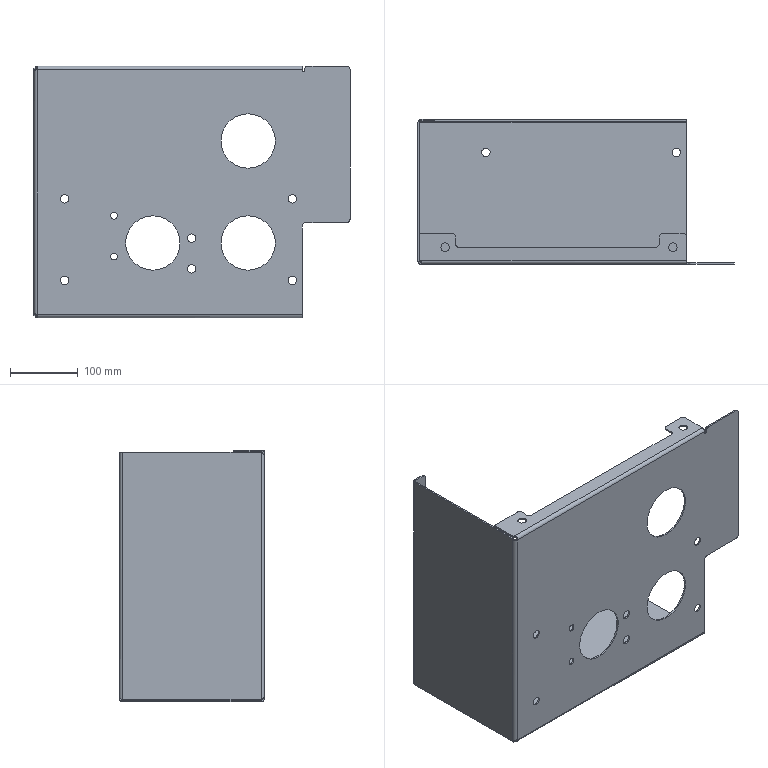Part | SolidWorks | features ICE 5, EdgeFlange 2, CornerRelief 1, Fillet 1, FlatPattern 1, SMBaseFlange 1, SheetMetal 1 | 1 solid | 113 faces | box 465 x 213 x 370 mm | volume 766424 mm3 | cylinder 60 | plane 43 | spline 10 | commonest cylinder face diameters 12.5 x24 10 x15 80 x6 0.1 x3 5 x3 9.6 x3